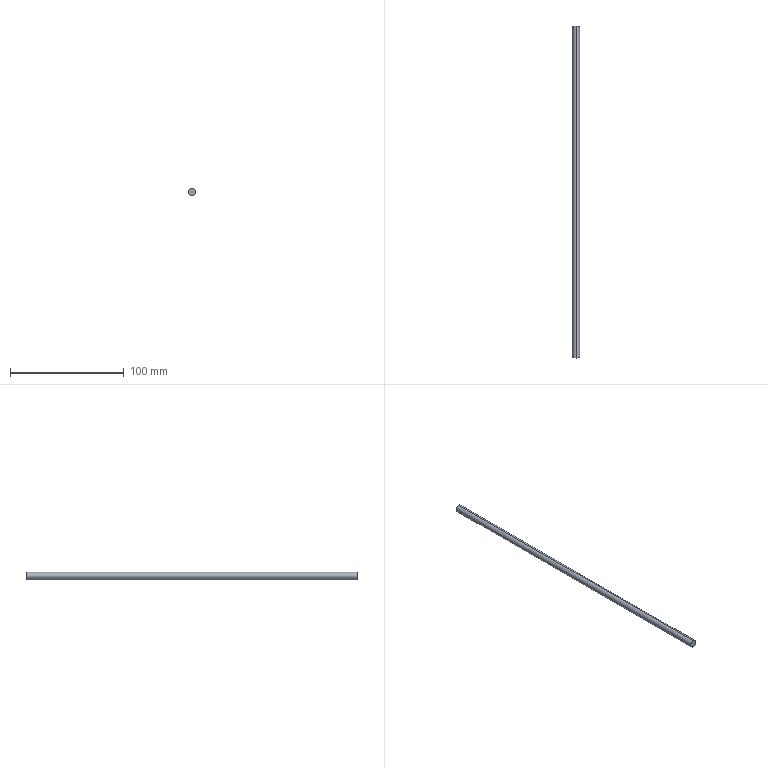Part | STEP file | 4-20.sldasm-Part-341 | 1 solid | 4 faces | box 6.35 x 292.067 x 6.35 mm | volume 9250 mm3 | cylinder 2 | plane 2 | commonest cylinder face diameters 6.35 x2
STEP:
#1=CARTESIAN_POINT('',(15.,357.067,113.175));
#2=VERTEX_POINT('',#1);
#3=CARTESIAN_POINT('',(15.,357.067,106.825));
#4=VERTEX_POINT('',#3);
#5=CARTESIAN_POINT('',(15.,357.067,110.));
#6=DIRECTION('',(0.,-1.,0.));
#7=DIRECTION('',(1.,0.,0.));
#8=AXIS2_PLACEMENT_3D('',#5,#6,#7);
#9=CIRCLE('',#8,3.175);
#10=EDGE_CURVE('',#2,#4,#9,.T.);
#11=ORIENTED_EDGE('',*,*,#10,.T.);
#12=CARTESIAN_POINT('',(15.,65.,106.825));
#13=VERTEX_POINT('',#12);
#14=CARTESIAN_POINT('',(15.,373.067,106.825));
#15=DIRECTION('',(0.,-1.,0.));
#16=VECTOR('',#15,1000.);
#17=LINE('',#14,#16);
#18=EDGE_CURVE('',#4,#13,#17,.T.);
#19=ORIENTED_EDGE('',*,*,#18,.T.);
#20=CARTESIAN_POINT('',(15.,65.,113.175));
#21=VERTEX_POINT('',#20);
#22=CARTESIAN_POINT('',(15.,65.,110.));
#23=DIRECTION('',(0.,1.,0.));
#24=DIRECTION('',(1.,0.,0.));
#25=AXIS2_PLACEMENT_3D('',#22,#23,#24);
#26=CIRCLE('',#25,3.175);
#27=EDGE_CURVE('',#13,#21,#26,.T.);
#28=ORIENTED_EDGE('',*,*,#27,.T.);
#29=CARTESIAN_POINT('',(15.,373.067,113.175));
#30=DIRECTION('',(0.,-1.,0.));
#31=VECTOR('',#30,1000.);
#32=LINE('',#29,#31);
#33=EDGE_CURVE('',#2,#21,#32,.T.);
#34=ORIENTED_EDGE('',*,*,#33,.F.);
#35=EDGE_LOOP('',(#11,#19,#28,#34));
#36=FACE_OUTER_BOUND('',#35,.T.);
#37=CARTESIAN_POINT('',(15.,373.067,110.));
#38=DIRECTION('',(0.,-1.,0.));
#39=DIRECTION('',(0.,0.,1.));
#40=AXIS2_PLACEMENT_3D('',#37,#38,#39);
#41=CYLINDRICAL_SURFACE('',#40,3.175);
#42=ADVANCED_FACE('',(#36),#41,.T.);
#43=CARTESIAN_POINT('',(15.,65.,110.));
#44=DIRECTION('',(0.,1.,0.));
#45=DIRECTION('',(1.,0.,0.));
#46=AXIS2_PLACEMENT_3D('',#43,#44,#45);
#47=CIRCLE('',#46,3.175);
#48=EDGE_CURVE('',#21,#13,#47,.T.);
#49=ORIENTED_EDGE('',*,*,#48,.F.);
#50=ORIENTED_EDGE('',*,*,#27,.F.);
#51=EDGE_LOOP('',(#49,#50));
#52=FACE_OUTER_BOUND('',#51,.T.);
#53=CARTESIAN_POINT('',(15.,65.,110.));
#54=DIRECTION('',(0.,1.,0.));
#55=DIRECTION('',(1.,0.,0.));
#56=AXIS2_PLACEMENT_3D('',#53,#54,#55);
#57=PLANE('',#56);
#58=ADVANCED_FACE('',(#52),#57,.F.);
#59=ORIENTED_EDGE('',*,*,#10,.F.);
#60=CARTESIAN_POINT('',(15.,357.067,110.));
#61=DIRECTION('',(0.,-1.,0.));
#62=DIRECTION('',(1.,0.,0.));
#63=AXIS2_PLACEMENT_3D('',#60,#61,#62);
#64=CIRCLE('',#63,3.175);
#65=EDGE_CURVE('',#4,#2,#64,.T.);
#66=ORIENTED_EDGE('',*,*,#65,.F.);
#67=EDGE_LOOP('',(#59,#66));
#68=FACE_OUTER_BOUND('',#67,.T.);
#69=CARTESIAN_POINT('',(15.,357.067,110.));
#70=DIRECTION('',(0.,1.,0.));
#71=DIRECTION('',(1.,0.,0.));
#72=AXIS2_PLACEMENT_3D('',#69,#70,#71);
#73=PLANE('',#72);
#74=ADVANCED_FACE('',(#68),#73,.T.);
#75=ORIENTED_EDGE('',*,*,#18,.F.);
#76=ORIENTED_EDGE('',*,*,#65,.T.);
#77=ORIENTED_EDGE('',*,*,#33,.T.);
#78=ORIENTED_EDGE('',*,*,#48,.T.);
#79=EDGE_LOOP('',(#75,#76,#77,#78));
#80=FACE_OUTER_BOUND('',#79,.T.);
#81=CARTESIAN_POINT('',(15.,373.067,110.));
#82=DIRECTION('',(0.,-1.,0.));
#83=DIRECTION('',(0.,0.,1.));
#84=AXIS2_PLACEMENT_3D('',#81,#82,#83);
#85=CYLINDRICAL_SURFACE('',#84,3.175);
#86=ADVANCED_FACE('',(#80),#85,.T.);
#87=CLOSED_SHELL('',(#42,#58,#74,#86));
#88=MANIFOLD_SOLID_BREP('',#87);
#89=CARTESIAN_POINT('',(0.,0.,0.));
#90=DIRECTION('',(0.,0.,1.));
#91=DIRECTION('',(1.,0.,0.));
#92=AXIS2_PLACEMENT_3D('',#89,#90,#91);
#93=(LENGTH_UNIT()NAMED_UNIT(*)SI_UNIT(.MILLI.,.METRE.));
#94=UNCERTAINTY_MEASURE_WITH_UNIT(LENGTH_MEASURE(0.00001),#93,'','');
#95=(NAMED_UNIT(*)PLANE_ANGLE_UNIT()SI_UNIT($,.RADIAN.));
#96=(NAMED_UNIT(*)SI_UNIT($,.STERADIAN.)SOLID_ANGLE_UNIT());
#97=(GEOMETRIC_REPRESENTATION_CONTEXT(3)GLOBAL_UNCERTAINTY_ASSIGNED_CONTEXT((#94))GLOBAL_UNIT_ASSIGNED_CONTEXT((#93,#95,#96))REPRESENTATION_CONTEXT('',''));
#98=ADVANCED_BREP_SHAPE_REPRESENTATION('',(#88,#92),#97);